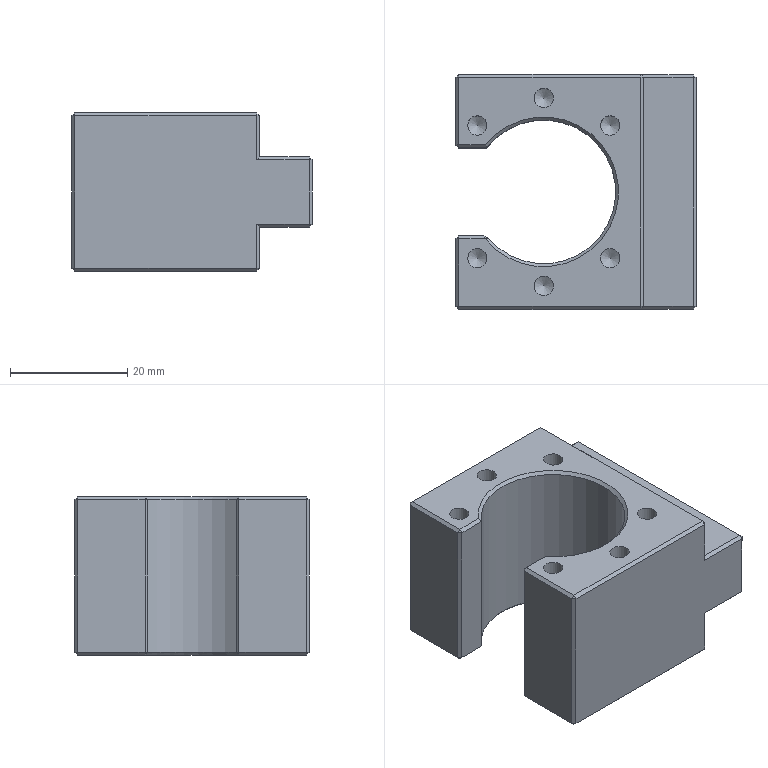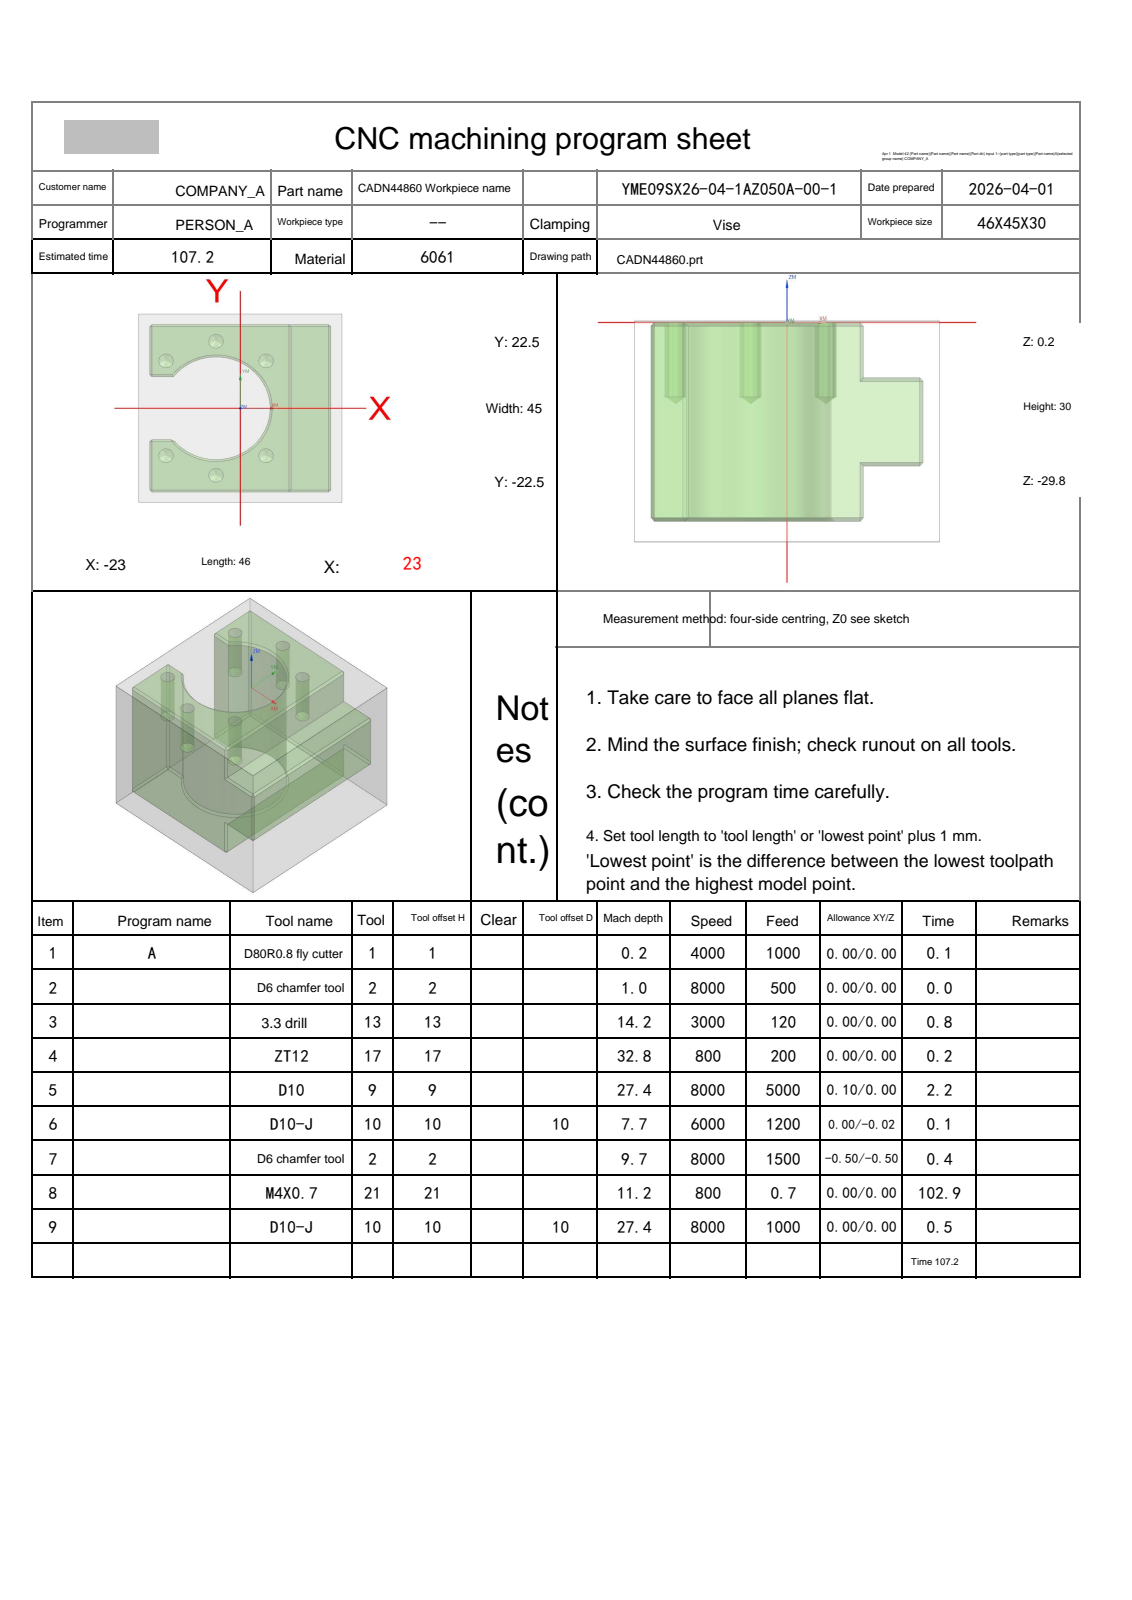NC program | NX | posted by the shop | part box 41 x 40 x 27 mm
Whole program, first 1134 of 1687 lines:
%
O0001
(Machine time: 203.22 MIN)
(===Total Tool:7===)
(T1=D80R0.8 fly cutter  D=80.  R=0.8  D-  H01 Z=-0.   )
(T2=D6 chamfer tool   D=6.   R=0.   D-  H02 Z=-9.5  )
(T13=3.3 drill  D=3.3  DR_a=118 D-  H13 Z=-14.  )
(T17=ZT12   D=12.  DR_a=118 D-  H17 Z=-32.61)
(T9=D10     D=10.  R=0.   D-  H09 Z=-27.2 )
(T10=D10-J  D=10.  R=0.   D10 H10 Z=-27.2 )
(T21=M4X0.7 D=3.3  DR_a=180 D-  H21 Z=-11.  )
G80 G90 G17 G49 G40
G91 G28 Z0
M01
N1 T01 M06
(D80R0.8 fly cutter D=80. R=0.8 H=01 ce=0.00 di=0.00)
G00 G90 G54 X-65.5 Y0.0 M03 S4000
G43 H01 Z20.
M08
Z2.
G01 Z0.0 F1000.
X-60.5
X60.5
X65.5
Z2.
G00 Z20.
G91 G28 Z0.0
M05
M09
G91 G28 Z0.0
M01
N2 T02 M06
(D6 chamfer tool D=6. R=0. H=02 ce=0.00 di=0.00)
G00 G90 G54 X-16.809 Y-11.314 M03 S8000
G43 H02 Z20.
M08
G98 G81 X-16.809 Y-11.314 Z-.8 R1. F500.
X-5.496 Y-16.
X5.818 Y-11.314
X-5.5 Y0.0
X-16.809 Y11.314
X-5.496 Y16.
X5.818 Y11.314
G80
G00 Z20.
G91 G28 Z0.0
M05
M09
G91 G28 Z0.0
M01
N3 T13 M06
(3.3 drill D=3.3 DR_a=118 H=13)
G00 G90 G54 X5.818 Y11.314 M03 S3000
G43 H13 Z20.
M08
G98 G83 X5.818 Y11.314 Z-14. R1. F120. Q2.
X-5.496 Y16.
X-16.809 Y11.314
Y-11.314
X-5.496 Y-16.
X5.818 Y-11.314
G80
G00 Z20.
G91 G28 Z0.0
M05
M09
G91 G28 Z0.0
M01
N4 T17 M06
(ZT12 D=12. DR_a=118 H=17)
G00 G90 G54 X-5.5 Y0.0 M03 S800
G43 H17 Z20.
M08
G98 G83 X-5.5 Y0.0 Z-32.605 R1. F200. Q3.
G80
G00 Z20.
G91 G28 Z0.0
M05
M09
G91 G28 Z0.0
M01
N5 T09 M06
(D10  D=10. R=0. H=09 ce=0.10 di=0.00)
G00 G90 G54 X0.0 Y-25.1 M03 S8000
G43 H09 Z20.
M08
Z.5
G01 X-20. Z.436 F5000.
G02 X-23.606 Y-23.606 Z.424 I0.0 J5.1
G01 X-24.106 Y-23.106 Z.421
G02 X-25.6 Y-19.5 Z.409 I3.606 J3.606
G01 Y-8. Z.372
G02 X-24.106 Y-4.394 Z.359 I5.1 J0.0
G01 X-23.606 Y-3.894 Z.357
G02 X-20. Y-2.4 Z.344 I3.606 J-3.606
G01 X-15.699 Z.331
G02 X-13.545 Y-2.877 Z.323 I0.0 J-5.1
G01 X-12.724 Y-3.26 Z.321
G02 X-10.973 Y-4.601 Z.314 I-2.153 J-4.623
G03 X-.899 Y-5.473 Z.278 I5.473 J4.601
X-.027 Y4.601 Z.242 I-4.601 J5.473
X-10.101 Y5.473 Z.206 I-5.473 J-4.601
X-11.153 Y4.378 Z.201 I4.601 J-5.473
G02 X-15.186 Y2.4 Z.187 I-4.032 J3.122
G01 X-20. Z.171
G02 X-23.606 Y3.894 Z.159 I0.0 J5.1
G01 X-24.106 Y4.394 Z.156
G02 X-25.6 Y8. Z.144 I3.606 J3.606
G01 Y19.5 Z.107
G02 X-24.106 Y23.106 Z.094 I5.1 J0.0
G01 X-23.606 Y23.606 Z.092
G02 X-20. Y25.1 Z.079 I3.606 J-3.606
G01 X20. Z-.048
G02 X23.606 Y23.606 Z-.061 I0.0 J-5.1
G01 X24.106 Y23.106 Z-.063
G02 X25.6 Y19.5 Z-.076 I-3.606 J-3.606
G01 Y-19.5 Z-.2
G02 X24.106 Y-23.106 Z-.213 I-5.1 J0.0
G01 X23.606 Y-23.606 Z-.215
G02 X20. Y-25.1 Z-.228 I-3.606 J3.606
G01 X-20. Z-.355
G02 X-23.606 Y-23.606 Z-.368 I0.0 J5.1
G01 X-24.106 Y-23.106 Z-.37
G02 X-25.6 Y-19.5 Z-.383 I3.606 J3.606
G01 Y-8. Z-.419
G02 X-24.106 Y-4.394 Z-.432 I5.1 J0.0
G01 X-23.606 Y-3.894 Z-.434
G02 X-20. Y-2.4 Z-.447 I3.606 J-3.606
G01 X-15.699 Z-.461
G02 X-13.545 Y-2.877 Z-.468 I0.0 J-5.1
G01 X-12.724 Y-3.26 Z-.471
G02 X-10.973 Y-4.601 Z-.478 I-2.153 J-4.623
G03 X-.899 Y-5.473 Z-.514 I5.473 J4.601
X-.027 Y4.601 Z-.549 I-4.601 J5.473
X-10.101 Y5.473 Z-.585 I-5.473 J-4.601
X-11.153 Y4.378 Z-.59 I4.601 J-5.473
G02 X-15.186 Y2.4 Z-.605 I-4.032 J3.122
G01 X-20. Z-.62
G02 X-23.606 Y3.894 Z-.633 I0.0 J5.1
G01 X-24.106 Y4.394 Z-.635
G02 X-25.6 Y8. Z-.648 I3.606 J3.606
G01 Y19.5 Z-.684
G02 X-24.106 Y23.106 Z-.697 I5.1 J0.0
G01 X-23.606 Y23.606 Z-.699
G02 X-20. Y25.1 Z-.712 I3.606 J-3.606
G01 X20. Z-.84
G02 X23.606 Y23.606 Z-.852 I0.0 J-5.1
G01 X24.106 Y23.106 Z-.855
G02 X25.6 Y19.5 Z-.867 I-3.606 J-3.606
G01 Y-19.5 Z-.991
G02 X24.106 Y-23.106 Z-1.004 I-5.1 J0.0
G01 X23.606 Y-23.606 Z-1.006
G02 X20. Y-25.1 Z-1.019 I-3.606 J3.606
G01 X-20. Z-1.147
G02 X-23.606 Y-23.606 Z-1.159 I0.0 J5.1
G01 X-24.106 Y-23.106 Z-1.162
G02 X-25.6 Y-19.5 Z-1.174 I3.606 J3.606
G01 Y-8. Z-1.211
G02 X-24.106 Y-4.394 Z-1.224 I5.1 J0.0
G01 X-23.606 Y-3.894 Z-1.226
G02 X-20. Y-2.4 Z-1.239 I3.606 J-3.606
G01 X-15.699 Z-1.252
G02 X-13.545 Y-2.877 Z-1.259 I0.0 J-5.1
G01 X-12.724 Y-3.26 Z-1.262
G02 X-10.973 Y-4.601 Z-1.269 I-2.153 J-4.623
G03 X-.899 Y-5.473 Z-1.305 I5.473 J4.601
X-.027 Y4.601 Z-1.341 I-4.601 J5.473
X-10.101 Y5.473 Z-1.377 I-5.473 J-4.601
X-11.153 Y4.378 Z-1.381 I4.601 J-5.473
G02 X-15.186 Y2.4 Z-1.396 I-4.032 J3.122
G01 X-20. Z-1.412
G02 X-23.606 Y3.894 Z-1.424 I0.0 J5.1
G01 X-24.106 Y4.394 Z-1.427
G02 X-25.6 Y8. Z-1.439 I3.606 J3.606
G01 Y19.5 Z-1.476
G02 X-24.106 Y23.106 Z-1.489 I5.1 J0.0
G01 X-23.606 Y23.606 Z-1.491
G02 X-20. Y25.1 Z-1.504 I3.606 J-3.606
G01 X20. Z-1.631
G02 X23.606 Y23.606 Z-1.644 I0.0 J-5.1
G01 X24.106 Y23.106 Z-1.646
G02 X25.6 Y19.5 Z-1.659 I-3.606 J-3.606
G01 Y-19.5 Z-1.783
G02 X24.106 Y-23.106 Z-1.796 I-5.1 J0.0
G01 X23.606 Y-23.606 Z-1.798
G02 X20. Y-25.1 Z-1.811 I-3.606 J3.606
G01 X-20. Z-1.938
G02 X-23.606 Y-23.606 Z-1.951 I0.0 J5.1
G01 X-24.106 Y-23.106 Z-1.953
G02 X-25.6 Y-19.5 Z-1.966 I3.606 J3.606
G01 Y-8. Z-2.002
G02 X-24.106 Y-4.394 Z-2.015 I5.1 J0.0
G01 X-23.606 Y-3.894 Z-2.017
G02 X-20. Y-2.4 Z-2.03 I3.606 J-3.606
G01 X-15.699 Z-2.044
G02 X-13.545 Y-2.877 Z-2.051 I0.0 J-5.1
G01 X-12.724 Y-3.26 Z-2.054
G02 X-10.973 Y-4.601 Z-2.061 I-2.153 J-4.623
G03 X-.899 Y-5.473 Z-2.097 I5.473 J4.601
X-.027 Y4.601 Z-2.132 I-4.601 J5.473
X-10.101 Y5.473 Z-2.168 I-5.473 J-4.601
X-11.153 Y4.378 Z-2.173 I4.601 J-5.473
G02 X-15.186 Y2.4 Z-2.188 I-4.032 J3.122
G01 X-20. Z-2.203
G02 X-23.606 Y3.894 Z-2.216 I0.0 J5.1
G01 X-24.106 Y4.394 Z-2.218
G02 X-25.6 Y8. Z-2.231 I3.606 J3.606
G01 Y19.5 Z-2.267
G02 X-24.106 Y23.106 Z-2.28 I5.1 J0.0
G01 X-23.606 Y23.606 Z-2.282
G02 X-20. Y25.1 Z-2.295 I3.606 J-3.606
G01 X20. Z-2.422
G02 X23.606 Y23.606 Z-2.435 I0.0 J-5.1
G01 X24.106 Y23.106 Z-2.437
G02 X25.6 Y19.5 Z-2.45 I-3.606 J-3.606
G01 Y-19.5 Z-2.574
G02 X24.106 Y-23.106 Z-2.587 I-5.1 J0.0
G01 X23.606 Y-23.606 Z-2.589
G02 X20. Y-25.1 Z-2.602 I-3.606 J3.606
G01 X-20. Z-2.729
G02 X-23.606 Y-23.606 Z-2.742 I0.0 J5.1
G01 X-24.106 Y-23.106 Z-2.744
G02 X-25.6 Y-19.5 Z-2.757 I3.606 J3.606
G01 Y-8. Z-2.794
G02 X-24.106 Y-4.394 Z-2.806 I5.1 J0.0
G01 X-23.606 Y-3.894 Z-2.809
G02 X-20. Y-2.4 Z-2.821 I3.606 J-3.606
G01 X-15.699 Z-2.835
G02 X-13.545 Y-2.877 Z-2.842 I0.0 J-5.1
G01 X-12.724 Y-3.26 Z-2.845
G02 X-10.973 Y-4.601 Z-2.852 I-2.153 J-4.623
G03 X-.899 Y-5.473 Z-2.888 I5.473 J4.601
X-.027 Y4.601 Z-2.924 I-4.601 J5.473
X-10.101 Y5.473 Z-2.959 I-5.473 J-4.601
X-11.153 Y4.378 Z-2.964 I4.601 J-5.473
G02 X-15.186 Y2.4 Z-2.979 I-4.032 J3.122
G01 X-20. Z-2.994
G02 X-23.606 Y3.894 Z-3.007 I0.0 J5.1
G01 X-24.106 Y4.394 Z-3.009
G02 X-25.6 Y8. Z-3.022 I3.606 J3.606
G01 Y19.5 Z-3.059
G02 X-24.106 Y23.106 Z-3.072 I5.1 J0.0
G01 X-23.606 Y23.606 Z-3.074
G02 X-20. Y25.1 Z-3.087 I3.606 J-3.606
G01 X20. Z-3.214
G02 X23.606 Y23.606 Z-3.227 I0.0 J-5.1
G01 X24.106 Y23.106 Z-3.229
G02 X25.6 Y19.5 Z-3.242 I-3.606 J-3.606
G01 Y-19.5 Z-3.366
G02 X24.106 Y-23.106 Z-3.378 I-5.1 J0.0
G01 X23.606 Y-23.606 Z-3.381
G02 X20. Y-25.1 Z-3.393 I-3.606 J3.606
G01 X-20. Z-3.521
G02 X-23.606 Y-23.606 Z-3.534 I0.0 J5.1
G01 X-24.106 Y-23.106 Z-3.536
G02 X-25.6 Y-19.5 Z-3.549 I3.606 J3.606
G01 Y-8. Z-3.585
G02 X-24.106 Y-4.394 Z-3.598 I5.1 J0.0
G01 X-23.606 Y-3.894 Z-3.6
G02 X-20. Y-2.4 Z-3.613 I3.606 J-3.606
G01 X-15.699 Z-3.627
G02 X-13.545 Y-2.877 Z-3.634 I0.0 J-5.1
G01 X-12.724 Y-3.26 Z-3.637
G02 X-10.973 Y-4.601 Z-3.644 I-2.153 J-4.623
G03 X-.899 Y-5.473 Z-3.679 I5.473 J4.601
X-.027 Y4.601 Z-3.715 I-4.601 J5.473
X-10.101 Y5.473 Z-3.751 I-5.473 J-4.601
X-11.153 Y4.378 Z-3.756 I4.601 J-5.473
G02 X-15.186 Y2.4 Z-3.771 I-4.032 J3.122
G01 X-20. Z-3.786
G02 X-23.606 Y3.894 Z-3.799 I0.0 J5.1
G01 X-24.106 Y4.394 Z-3.801
G02 X-25.6 Y8. Z-3.814 I3.606 J3.606
G01 Y19.5 Z-3.85
G02 X-24.106 Y23.106 Z-3.863 I5.1 J0.0
G01 X-23.606 Y23.606 Z-3.865
G02 X-20. Y25.1 Z-3.878 I3.606 J-3.606
G01 X20. Z-4.005
G02 X23.606 Y23.606 Z-4.018 I0.0 J-5.1
G01 X24.106 Y23.106 Z-4.02
G02 X25.6 Y19.5 Z-4.033 I-3.606 J-3.606
G01 Y-19.5 Z-4.157
G02 X24.106 Y-23.106 Z-4.17 I-5.1 J0.0
G01 X23.606 Y-23.606 Z-4.172
G02 X20. Y-25.1 Z-4.185 I-3.606 J3.606
G01 X-20. Z-4.312
G02 X-23.606 Y-23.606 Z-4.325 I0.0 J5.1
G01 X-24.106 Y-23.106 Z-4.327
G02 X-25.6 Y-19.5 Z-4.34 I3.606 J3.606
G01 Y-8. Z-4.377
G02 X-24.106 Y-4.394 Z-4.389 I5.1 J0.0
G01 X-23.606 Y-3.894 Z-4.392
G02 X-20. Y-2.4 Z-4.404 I3.606 J-3.606
G01 X-15.699 Z-4.418
G02 X-13.545 Y-2.877 Z-4.425 I0.0 J-5.1
G01 X-12.724 Y-3.26 Z-4.428
G02 X-10.973 Y-4.601 Z-4.435 I-2.153 J-4.623
G03 X-.899 Y-5.473 Z-4.471 I5.473 J4.601
X-.027 Y4.601 Z-4.507 I-4.601 J5.473
X-10.101 Y5.473 Z-4.542 I-5.473 J-4.601
X-11.153 Y4.378 Z-4.547 I4.601 J-5.473
G02 X-15.186 Y2.4 Z-4.562 I-4.032 J3.122
G01 X-20. Z-4.577
G02 X-23.606 Y3.894 Z-4.59 I0.0 J5.1
G01 X-24.106 Y4.394 Z-4.592
G02 X-25.6 Y8. Z-4.605 I3.606 J3.606
G01 Y19.5 Z-4.642
G02 X-24.106 Y23.106 Z-4.654 I5.1 J0.0
G01 X-23.606 Y23.606 Z-4.657
G02 X-20. Y25.1 Z-4.669 I3.606 J-3.606
G01 X20. Z-4.797
G02 X23.606 Y23.606 Z-4.809 I0.0 J-5.1
G01 X24.106 Y23.106 Z-4.812
G02 X25.6 Y19.5 Z-4.824 I-3.606 J-3.606
G01 Y-19.5 Z-4.949
G02 X24.106 Y-23.106 Z-4.961 I-5.1 J0.0
G01 X23.606 Y-23.606 Z-4.964
G02 X20. Y-25.1 Z-4.976 I-3.606 J3.606
G01 X-20. Z-5.104
G02 X-23.606 Y-23.606 Z-5.116 I0.0 J5.1
G01 X-24.106 Y-23.106 Z-5.119
G02 X-25.6 Y-19.5 Z-5.131 I3.606 J3.606
G01 Y-8. Z-5.168
G02 X-24.106 Y-4.394 Z-5.181 I5.1 J0.0
G01 X-23.606 Y-3.894 Z-5.183
G02 X-20. Y-2.4 Z-5.196 I3.606 J-3.606
G01 X-15.699 Z-5.209
G02 X-13.545 Y-2.877 Z-5.217 I0.0 J-5.1
G01 X-12.724 Y-3.26 Z-5.219
G02 X-10.973 Y-4.601 Z-5.226 I-2.153 J-4.623
G03 X-.899 Y-5.473 Z-5.262 I5.473 J4.601
X-.027 Y4.601 Z-5.298 I-4.601 J5.473
X-10.101 Y5.473 Z-5.334 I-5.473 J-4.601
X-11.153 Y4.378 Z-5.339 I4.601 J-5.473
G02 X-15.186 Y2.4 Z-5.353 I-4.032 J3.122
G01 X-20. Z-5.369
G02 X-23.606 Y3.894 Z-5.381 I0.0 J5.1
G01 X-24.106 Y4.394 Z-5.384
G02 X-25.6 Y8. Z-5.396 I3.606 J3.606
G01 Y19.5 Z-5.433
G02 X-24.106 Y23.106 Z-5.446 I5.1 J0.0
G01 X-23.606 Y23.606 Z-5.448
G02 X-20. Y25.1 Z-5.461 I3.606 J-3.606
G01 X20. Z-5.588
G02 X23.606 Y23.606 Z-5.601 I0.0 J-5.1
G01 X24.106 Y23.106 Z-5.603
G02 X25.6 Y19.5 Z-5.616 I-3.606 J-3.606
G01 Y-19.5 Z-5.74
G02 X24.106 Y-23.106 Z-5.753 I-5.1 J0.0
G01 X23.606 Y-23.606 Z-5.755
G02 X20. Y-25.1 Z-5.768 I-3.606 J3.606
G01 X-20. Z-5.895
G02 X-23.606 Y-23.606 Z-5.908 I0.0 J5.1
G01 X-24.106 Y-23.106 Z-5.91
G02 X-25.6 Y-19.5 Z-5.923 I3.606 J3.606
G01 Y-8. Z-5.959
G02 X-24.106 Y-4.394 Z-5.972 I5.1 J0.0
G01 X-23.606 Y-3.894 Z-5.974
G02 X-20. Y-2.4 Z-5.987 I3.606 J-3.606
G01 X-15.699 Z-6.001
G02 X-13.545 Y-2.877 Z-6.008 I0.0 J-5.1
G01 X-12.724 Y-3.26 Z-6.011
G02 X-10.973 Y-4.601 Z-6.018 I-2.153 J-4.623
G03 X-.899 Y-5.473 Z-6.054 I5.473 J4.601
X-.027 Y4.601 Z-6.089 I-4.601 J5.473
X-10.101 Y5.473 Z-6.125 I-5.473 J-4.601
X-11.153 Y4.378 Z-6.13 I4.601 J-5.473
G02 X-15.186 Y2.4 Z-6.145 I-4.032 J3.122
G01 X-20. Z-6.16
G02 X-23.606 Y3.894 Z-6.173 I0.0 J5.1
G01 X-24.106 Y4.394 Z-6.175
G02 X-25.6 Y8. Z-6.188 I3.606 J3.606
G01 Y19.5 Z-6.224
G02 X-24.106 Y23.106 Z-6.237 I5.1 J0.0
G01 X-23.606 Y23.606 Z-6.239
G02 X-20. Y25.1 Z-6.252 I3.606 J-3.606
G01 X20. Z-6.38
G02 X23.606 Y23.606 Z-6.392 I0.0 J-5.1
G01 X24.106 Y23.106 Z-6.395
G02 X25.6 Y19.5 Z-6.407 I-3.606 J-3.606
G01 Y-19.5 Z-6.531
G02 X24.106 Y-23.106 Z-6.544 I-5.1 J0.0
G01 X23.606 Y-23.606 Z-6.546
G02 X20. Y-25.1 Z-6.559 I-3.606 J3.606
G01 X-20. Z-6.687
G02 X-23.606 Y-23.606 Z-6.699 I0.0 J5.1
G01 X-24.106 Y-23.106 Z-6.702
G02 X-25.6 Y-19.5 Z-6.714 I3.606 J3.606
G01 Y-8. Z-6.751
G02 X-24.106 Y-4.394 Z-6.764 I5.1 J0.0
G01 X-23.606 Y-3.894 Z-6.766
G02 X-20. Y-2.4 Z-6.779 I3.606 J-3.606
G01 X-15.699 Z-6.792
G02 X-13.545 Y-2.877 Z-6.799 I0.0 J-5.1
G01 X-12.724 Y-3.26 Z-6.802
G02 X-10.973 Y-4.601 Z-6.809 I-2.153 J-4.623
G03 X-.899 Y-5.473 Z-6.845 I5.473 J4.601
X-.027 Y4.601 Z-6.881 I-4.601 J5.473
X-10.101 Y5.473 Z-6.917 I-5.473 J-4.601
X-11.153 Y4.378 Z-6.921 I4.601 J-5.473
G02 X-15.186 Y2.4 Z-6.936 I-4.032 J3.122
G01 X-20. Z-6.952
G02 X-23.606 Y3.894 Z-6.964 I0.0 J5.1
G01 X-24.106 Y4.394 Z-6.967
G02 X-25.6 Y8. Z-6.979 I3.606 J3.606
G01 Y19.5 Z-7.016
G02 X-24.106 Y23.106 Z-7.029 I5.1 J0.0
G01 X-23.606 Y23.606 Z-7.031
G02 X-20. Y25.1 Z-7.044 I3.606 J-3.606
G01 X20. Z-7.171
G02 X23.606 Y23.606 Z-7.184 I0.0 J-5.1
G01 X24.106 Y23.106 Z-7.186
G02 X25.6 Y19.5 Z-7.199 I-3.606 J-3.606
G01 Y-19.5 Z-7.323
G02 X24.106 Y-23.106 Z-7.336 I-5.1 J0.0
G01 X23.606 Y-23.606 Z-7.338
G02 X20. Y-25.1 Z-7.351 I-3.606 J3.606
G01 X-20. Z-7.478
G02 X-23.606 Y-23.606 Z-7.491 I0.0 J5.1
G01 X-24.106 Y-23.106 Z-7.493
G02 X-25.6 Y-19.5 Z-7.506 I3.606 J3.606
G01 Y-8. Z-7.542
G02 X-24.106 Y-4.394 Z-7.555 I5.1 J0.0
G01 X-23.606 Y-3.894 Z-7.557
G02 X-20. Y-2.4 Z-7.57 I3.606 J-3.606
G01 X-15.699 Z-7.584
G02 X-13.545 Y-2.877 Z-7.591 I0.0 J-5.1
G01 X-12.724 Y-3.26 Z-7.594
G02 X-10.973 Y-4.601 Z-7.601 I-2.153 J-4.623
G03 X-.899 Y-5.473 Z-7.637 I5.473 J4.601
X-.027 Y4.601 Z-7.672 I-4.601 J5.473
X-10.101 Y5.473 Z-7.708 I-5.473 J-4.601
X-11.153 Y4.378 Z-7.713 I4.601 J-5.473
G02 X-15.186 Y2.4 Z-7.728 I-4.032 J3.122
G01 X-20. Z-7.743
G02 X-23.606 Y3.894 Z-7.756 I0.0 J5.1
G01 X-24.106 Y4.394 Z-7.758
G02 X-25.6 Y8. Z-7.771 I3.606 J3.606
G01 Y19.5 Z-7.807
G02 X-24.106 Y23.106 Z-7.82 I5.1 J0.0
G01 X-23.606 Y23.606 Z-7.822
G02 X-20. Y25.1 Z-7.835 I3.606 J-3.606
G01 X20. Z-7.962
G02 X23.606 Y23.606 Z-7.975 I0.0 J-5.1
G01 X24.106 Y23.106 Z-7.977
G02 X25.6 Y19.5 Z-7.99 I-3.606 J-3.606
G01 Y-19.5 Z-8.114
G02 X24.106 Y-23.106 Z-8.127 I-5.1 J0.0
G01 X23.606 Y-23.606 Z-8.129
G02 X20. Y-25.1 Z-8.142 I-3.606 J3.606
G01 X-20. Z-8.269
G02 X-23.606 Y-23.606 Z-8.282 I0.0 J5.1
G01 X-24.106 Y-23.106 Z-8.284
G02 X-25.6 Y-19.5 Z-8.297 I3.606 J3.606
G01 Y-8. Z-8.334
G02 X-24.106 Y-4.394 Z-8.346 I5.1 J0.0
G01 X-23.606 Y-3.894 Z-8.349
G02 X-20. Y-2.4 Z-8.361 I3.606 J-3.606
G01 X-15.699 Z-8.375
G02 X-13.545 Y-2.877 Z-8.382 I0.0 J-5.1
G01 X-12.724 Y-3.26 Z-8.385
G02 X-10.973 Y-4.601 Z-8.392 I-2.153 J-4.623
G03 X-.899 Y-5.473 Z-8.428 I5.473 J4.601
X-.027 Y4.601 Z-8.464 I-4.601 J5.473
X-10.101 Y5.473 Z-8.499 I-5.473 J-4.601
X-11.153 Y4.378 Z-8.504 I4.601 J-5.473
G02 X-15.186 Y2.4 Z-8.519 I-4.032 J3.122
G01 X-20. Z-8.534
G02 X-23.606 Y3.894 Z-8.547 I0.0 J5.1
G01 X-24.106 Y4.394 Z-8.549
G02 X-25.6 Y8. Z-8.562 I3.606 J3.606
G01 Y19.5 Z-8.599
G02 X-24.106 Y23.106 Z-8.612 I5.1 J0.0
G01 X-23.606 Y23.606 Z-8.614
G02 X-20. Y25.1 Z-8.627 I3.606 J-3.606
G01 X20. Z-8.754
G02 X23.606 Y23.606 Z-8.767 I0.0 J-5.1
G01 X24.106 Y23.106 Z-8.769
G02 X25.6 Y19.5 Z-8.782 I-3.606 J-3.606
G01 Y-19.5 Z-8.906
G02 X24.106 Y-23.106 Z-8.918 I-5.1 J0.0
G01 X23.606 Y-23.606 Z-8.921
G02 X20. Y-25.1 Z-8.933 I-3.606 J3.606
G01 X-20. Z-9.061
G02 X-23.606 Y-23.606 Z-9.074 I0.0 J5.1
G01 X-24.106 Y-23.106 Z-9.076
G02 X-25.6 Y-19.5 Z-9.089 I3.606 J3.606
G01 Y-8. Z-9.125
G02 X-24.106 Y-4.394 Z-9.138 I5.1 J0.0
G01 X-23.606 Y-3.894 Z-9.14
G02 X-20. Y-2.4 Z-9.153 I3.606 J-3.606
G01 X-15.699 Z-9.167
G02 X-13.545 Y-2.877 Z-9.174 I0.0 J-5.1
G01 X-12.724 Y-3.26 Z-9.177
G02 X-10.973 Y-4.601 Z-9.184 I-2.153 J-4.623
G03 X-.899 Y-5.473 Z-9.219 I5.473 J4.601
X-.027 Y4.601 Z-9.255 I-4.601 J5.473
X-10.101 Y5.473 Z-9.291 I-5.473 J-4.601
X-11.153 Y4.378 Z-9.296 I4.601 J-5.473
G02 X-15.186 Y2.4 Z-9.311 I-4.032 J3.122
G01 X-20. Z-9.326
G02 X-23.606 Y3.894 Z-9.339 I0.0 J5.1
G01 X-24.106 Y4.394 Z-9.341
G02 X-25.6 Y8. Z-9.354 I3.606 J3.606
G01 Y19.5 Z-9.39
G02 X-24.106 Y23.106 Z-9.403 I5.1 J0.0
G01 X-23.606 Y23.606 Z-9.405
G02 X-20. Y25.1 Z-9.418 I3.606 J-3.606
G01 X20. Z-9.545
G02 X23.606 Y23.606 Z-9.558 I0.0 J-5.1
G01 X24.106 Y23.106 Z-9.56
G02 X25.6 Y19.5 Z-9.573 I-3.606 J-3.606
G01 Y-19.5 Z-9.697
G02 X24.106 Y-23.106 Z-9.71 I-5.1 J0.0
G01 X23.606 Y-23.606 Z-9.712
G02 X20. Y-25.1 Z-9.725 I-3.606 J3.606
G01 X-20. Z-9.852
G02 X-23.606 Y-23.606 Z-9.865 I0.0 J5.1
G01 X-24.106 Y-23.106 Z-9.867
G02 X-25.6 Y-19.5 Z-9.88 I3.606 J3.606
G01 Y-8. Z-9.917
G02 X-24.106 Y-4.394 Z-9.929 I5.1 J0.0
G01 X-23.606 Y-3.894 Z-9.932
G02 X-20. Y-2.4 Z-9.944 I3.606 J-3.606
G01 X-15.699 Z-9.958
G02 X-13.545 Y-2.877 Z-9.965 I0.0 J-5.1
G01 X-12.724 Y-3.26 Z-9.968
G02 X-10.973 Y-4.601 Z-9.975 I-2.153 J-4.623
G03 X-.899 Y-5.473 Z-10.011 I5.473 J4.601
X-.027 Y4.601 Z-10.047 I-4.601 J5.473
X-10.101 Y5.473 Z-10.082 I-5.473 J-4.601
X-11.153 Y4.378 Z-10.087 I4.601 J-5.473
G02 X-15.186 Y2.4 Z-10.102 I-4.032 J3.122
G01 X-20. Z-10.117
G02 X-23.606 Y3.894 Z-10.13 I0.0 J5.1
G01 X-24.106 Y4.394 Z-10.132
G02 X-25.6 Y8. Z-10.145 I3.606 J3.606
G01 Y19.5 Z-10.182
G02 X-24.106 Y23.106 Z-10.194 I5.1 J0.0
G01 X-23.606 Y23.606 Z-10.197
G02 X-20. Y25.1 Z-10.209 I3.606 J-3.606
G01 X20. Z-10.337
G02 X23.606 Y23.606 Z-10.349 I0.0 J-5.1
G01 X24.106 Y23.106 Z-10.352
G02 X25.6 Y19.5 Z-10.364 I-3.606 J-3.606
G01 Y-19.5 Z-10.489
G02 X24.106 Y-23.106 Z-10.501 I-5.1 J0.0
G01 X23.606 Y-23.606 Z-10.504
G02 X20. Y-25.1 Z-10.516 I-3.606 J3.606
G01 X-20. Z-10.644
G02 X-23.606 Y-23.606 Z-10.656 I0.0 J5.1
G01 X-24.106 Y-23.106 Z-10.659
G02 X-25.6 Y-19.5 Z-10.671 I3.606 J3.606
G01 Y-8. Z-10.708
G02 X-24.106 Y-4.394 Z-10.721 I5.1 J0.0
G01 X-23.606 Y-3.894 Z-10.723
G02 X-20. Y-2.4 Z-10.736 I3.606 J-3.606
G01 X-15.699 Z-10.749
G02 X-13.545 Y-2.877 Z-10.757 I0.0 J-5.1
G01 X-12.724 Y-3.26 Z-10.759
G02 X-10.973 Y-4.601 Z-10.766 I-2.153 J-4.623
G03 X-.899 Y-5.473 Z-10.802 I5.473 J4.601
X-.027 Y4.601 Z-10.838 I-4.601 J5.473
X-10.101 Y5.473 Z-10.874 I-5.473 J-4.601
X-11.153 Y4.378 Z-10.879 I4.601 J-5.473
G02 X-15.186 Y2.4 Z-10.893 I-4.032 J3.122
G01 X-20. Z-10.909
G02 X-23.606 Y3.894 Z-10.921 I0.0 J5.1
G01 X-24.106 Y4.394 Z-10.924
G02 X-25.6 Y8. Z-10.936 I3.606 J3.606
G01 Y19.5 Z-10.973
G02 X-24.106 Y23.106 Z-10.986 I5.1 J0.0
G01 X-23.606 Y23.606 Z-10.988
G02 X-20. Y25.1 Z-11.001 I3.606 J-3.606
G01 X20. Z-11.128
G02 X23.606 Y23.606 Z-11.141 I0.0 J-5.1
G01 X24.106 Y23.106 Z-11.143
G02 X25.6 Y19.5 Z-11.156 I-3.606 J-3.606
G01 Y-19.5 Z-11.28
G02 X24.106 Y-23.106 Z-11.293 I-5.1 J0.0
G01 X23.606 Y-23.606 Z-11.295
G02 X20. Y-25.1 Z-11.308 I-3.606 J3.606
G01 X-20. Z-11.435
G02 X-23.606 Y-23.606 Z-11.448 I0.0 J5.1
G01 X-24.106 Y-23.106 Z-11.45
G02 X-25.6 Y-19.5 Z-11.463 I3.606 J3.606
G01 Y-8. Z-11.499
G02 X-24.106 Y-4.394 Z-11.512 I5.1 J0.0
G01 X-23.606 Y-3.894 Z-11.514
G02 X-20. Y-2.4 Z-11.527 I3.606 J-3.606
G01 X-15.699 Z-11.541
G02 X-13.545 Y-2.877 Z-11.548 I0.0 J-5.1
G01 X-12.724 Y-3.26 Z-11.551
G02 X-10.973 Y-4.601 Z-11.558 I-2.153 J-4.623
G03 X-.899 Y-5.473 Z-11.594 I5.473 J4.601
X-.027 Y4.601 Z-11.629 I-4.601 J5.473
X-10.101 Y5.473 Z-11.665 I-5.473 J-4.601
X-11.153 Y4.378 Z-11.67 I4.601 J-5.473
G02 X-15.186 Y2.4 Z-11.685 I-4.032 J3.122
G01 X-20. Z-11.7
G02 X-23.606 Y3.894 Z-11.713 I0.0 J5.1
G01 X-24.106 Y4.394 Z-11.715
G02 X-25.6 Y8. Z-11.728 I3.606 J3.606
G01 Y19.5 Z-11.764
G02 X-24.106 Y23.106 Z-11.777 I5.1 J0.0
G01 X-23.606 Y23.606 Z-11.779
G02 X-20. Y25.1 Z-11.792 I3.606 J-3.606
G01 X20. Z-11.92
G02 X23.606 Y23.606 Z-11.932 I0.0 J-5.1
G01 X24.106 Y23.106 Z-11.935
G02 X25.6 Y19.5 Z-11.947 I-3.606 J-3.606
G01 Y-19.5 Z-12.071
G02 X24.106 Y-23.106 Z-12.084 I-5.1 J0.0
G01 X23.606 Y-23.606 Z-12.086
G02 X20. Y-25.1 Z-12.099 I-3.606 J3.606
G01 X-20. Z-12.227
G02 X-23.606 Y-23.606 Z-12.239 I0.0 J5.1
G01 X-24.106 Y-23.106 Z-12.242
G02 X-25.6 Y-19.5 Z-12.254 I3.606 J3.606
G01 Y-8. Z-12.291
G02 X-24.106 Y-4.394 Z-12.304 I5.1 J0.0
G01 X-23.606 Y-3.894 Z-12.306
G02 X-20. Y-2.4 Z-12.319 I3.606 J-3.606
G01 X-15.699 Z-12.332
G02 X-13.545 Y-2.877 Z-12.339 I0.0 J-5.1
G01 X-12.724 Y-3.26 Z-12.342
G02 X-10.973 Y-4.601 Z-12.349 I-2.153 J-4.623
G03 X-.899 Y-5.473 Z-12.385 I5.473 J4.601
X-.027 Y4.601 Z-12.421 I-4.601 J5.473
X-10.101 Y5.473 Z-12.457 I-5.473 J-4.601
X-11.153 Y4.378 Z-12.461 I4.601 J-5.473
G02 X-15.186 Y2.4 Z-12.476 I-4.032 J3.122
G01 X-20. Z-12.492
G02 X-23.606 Y3.894 Z-12.504 I0.0 J5.1
G01 X-24.106 Y4.394 Z-12.507
G02 X-25.6 Y8. Z-12.519 I3.606 J3.606
G01 Y19.5 Z-12.556
G02 X-24.106 Y23.106 Z-12.569 I5.1 J0.0
G01 X-23.606 Y23.606 Z-12.571
G02 X-20. Y25.1 Z-12.584 I3.606 J-3.606
G01 X20. Z-12.711
G02 X23.606 Y23.606 Z-12.724 I0.0 J-5.1
G01 X24.106 Y23.106 Z-12.726
G02 X25.6 Y19.5 Z-12.739 I-3.606 J-3.606
G01 Y-19.5 Z-12.863
G02 X24.106 Y-23.106 Z-12.876 I-5.1 J0.0
G01 X23.606 Y-23.606 Z-12.878
G02 X20. Y-25.1 Z-12.891 I-3.606 J3.606
G01 X-20. Z-13.018
G02 X-23.606 Y-23.606 Z-13.031 I0.0 J5.1
G01 X-24.106 Y-23.106 Z-13.033
G02 X-25.6 Y-19.5 Z-13.046 I3.606 J3.606
G01 Y-8. Z-13.082
G02 X-24.106 Y-4.394 Z-13.095 I5.1 J0.0
G01 X-23.606 Y-3.894 Z-13.097
G02 X-20. Y-2.4 Z-13.11 I3.606 J-3.606
G01 X-15.699 Z-13.124
G02 X-13.545 Y-2.877 Z-13.131 I0.0 J-5.1
G01 X-12.724 Y-3.26 Z-13.134
G02 X-10.973 Y-4.601 Z-13.141 I-2.153 J-4.623
G03 X-.899 Y-5.473 Z-13.177 I5.473 J4.601
X-.027 Y4.601 Z-13.212 I-4.601 J5.473
X-10.101 Y5.473 Z-13.248 I-5.473 J-4.601
X-11.153 Y4.378 Z-13.253 I4.601 J-5.473
G02 X-15.186 Y2.4 Z-13.268 I-4.032 J3.122
G01 X-20. Z-13.283
G02 X-23.606 Y3.894 Z-13.296 I0.0 J5.1
G01 X-24.106 Y4.394 Z-13.298
G02 X-25.6 Y8. Z-13.311 I3.606 J3.606
G01 Y19.5 Z-13.347
G02 X-24.106 Y23.106 Z-13.36 I5.1 J0.0
G01 X-23.606 Y23.606 Z-13.362
G02 X-20. Y25.1 Z-13.375 I3.606 J-3.606
G01 X20. Z-13.502
G02 X23.606 Y23.606 Z-13.515 I0.0 J-5.1
G01 X24.106 Y23.106 Z-13.517
G02 X25.6 Y19.5 Z-13.53 I-3.606 J-3.606
G01 Y-19.5 Z-13.654
G02 X24.106 Y-23.106 Z-13.667 I-5.1 J0.0
G01 X23.606 Y-23.606 Z-13.669
G02 X20. Y-25.1 Z-13.682 I-3.606 J3.606
G01 X-20. Z-13.809
G02 X-23.606 Y-23.606 Z-13.822 I0.0 J5.1
G01 X-24.106 Y-23.106 Z-13.824
G02 X-25.6 Y-19.5 Z-13.837 I3.606 J3.606
G01 Y-8. Z-13.874
G02 X-24.106 Y-4.394 Z-13.886 I5.1 J0.0
G01 X-23.606 Y-3.894 Z-13.889
G02 X-20. Y-2.4 Z-13.901 I3.606 J-3.606
G01 X-15.699 Z-13.915
G02 X-13.545 Y-2.877 Z-13.922 I0.0 J-5.1
G01 X-12.724 Y-3.26 Z-13.925
G02 X-10.973 Y-4.601 Z-13.932 I-2.153 J-4.623
G03 X-.899 Y-5.473 Z-13.968 I5.473 J4.601
X-.027 Y4.601 Z-14.004 I-4.601 J5.473
X-10.101 Y5.473 Z-14.039 I-5.473 J-4.601
X-11.153 Y4.378 Z-14.044 I4.601 J-5.473
G02 X-15.186 Y2.4 Z-14.059 I-4.032 J3.122
G01 X-20. Z-14.074
G02 X-23.606 Y3.894 Z-14.087 I0.0 J5.1
G01 X-24.106 Y4.394 Z-14.089
G02 X-25.6 Y8. Z-14.102 I3.606 J3.606
G01 Y19.5 Z-14.139
G02 X-24.106 Y23.106 Z-14.152 I5.1 J0.0
G01 X-23.606 Y23.606 Z-14.154
G02 X-20. Y25.1 Z-14.167 I3.606 J-3.606
G01 X20. Z-14.294
G02 X23.606 Y23.606 Z-14.307 I0.0 J-5.1
G01 X24.106 Y23.106 Z-14.309
G02 X25.6 Y19.5 Z-14.322 I-3.606 J-3.606
G01 Y-19.5 Z-14.446
G02 X24.106 Y-23.106 Z-14.458 I-5.1 J0.0
G01 X23.606 Y-23.606 Z-14.461
G02 X20. Y-25.1 Z-14.473 I-3.606 J3.606
G01 X-20. Z-14.601
G02 X-23.606 Y-23.606 Z-14.614 I0.0 J5.1
G01 X-24.106 Y-23.106 Z-14.616
G02 X-25.6 Y-19.5 Z-14.629 I3.606 J3.606
G01 Y-8. Z-14.665
G02 X-24.106 Y-4.394 Z-14.678 I5.1 J0.0
G01 X-23.606 Y-3.894 Z-14.68
G02 X-20. Y-2.4 Z-14.693 I3.606 J-3.606
G01 X-15.699 Z-14.707
G02 X-13.545 Y-2.877 Z-14.714 I0.0 J-5.1
G01 X-12.724 Y-3.26 Z-14.717
G02 X-10.973 Y-4.601 Z-14.724 I-2.153 J-4.623
G03 X-.899 Y-5.473 Z-14.759 I5.473 J4.601
X-.027 Y4.601 Z-14.795 I-4.601 J5.473
X-10.101 Y5.473 Z-14.831 I-5.473 J-4.601
X-11.153 Y4.378 Z-14.836 I4.601 J-5.473
G02 X-15.186 Y2.4 Z-14.851 I-4.032 J3.122
G01 X-20. Z-14.866
G02 X-23.606 Y3.894 Z-14.879 I0.0 J5.1
G01 X-24.106 Y4.394 Z-14.881
G02 X-25.6 Y8. Z-14.894 I3.606 J3.606
G01 Y19.5 Z-14.93
G02 X-24.106 Y23.106 Z-14.943 I5.1 J0.0
G01 X-23.606 Y23.606 Z-14.945
G02 X-20. Y25.1 Z-14.958 I3.606 J-3.606
G01 X20. Z-15.085
G02 X23.606 Y23.606 Z-15.098 I0.0 J-5.1
G01 X24.106 Y23.106 Z-15.1
G02 X25.6 Y19.5 Z-15.113 I-3.606 J-3.606
G01 Y-19.5 Z-15.237
G02 X24.106 Y-23.106 Z-15.25 I-5.1 J0.0
G01 X23.606 Y-23.606 Z-15.252
G02 X20. Y-25.1 Z-15.265 I-3.606 J3.606
G01 X-20. Z-15.392
G02 X-23.606 Y-23.606 Z-15.405 I0.0 J5.1
G01 X-24.106 Y-23.106 Z-15.407
G02 X-25.6 Y-19.5 Z-15.42 I3.606 J3.606
G01 Y-8. Z-15.457
G02 X-24.106 Y-4.394 Z-15.469 I5.1 J0.0
G01 X-23.606 Y-3.894 Z-15.472
G02 X-20. Y-2.4 Z-15.484 I3.606 J-3.606
G01 X-15.699 Z-15.498
G02 X-13.545 Y-2.877 Z-15.505 I0.0 J-5.1
G01 X-12.724 Y-3.26 Z-15.508
G02 X-10.973 Y-4.601 Z-15.515 I-2.153 J-4.623
G03 X-.899 Y-5.473 Z-15.551 I5.473 J4.601
X-.027 Y4.601 Z-15.587 I-4.601 J5.473
X-10.101 Y5.473 Z-15.622 I-5.473 J-4.601
X-11.153 Y4.378 Z-15.627 I4.601 J-5.473
G02 X-15.186 Y2.4 Z-15.642 I-4.032 J3.122
G01 X-20. Z-15.657
G02 X-23.606 Y3.894 Z-15.67 I0.0 J5.1
G01 X-24.106 Y4.394 Z-15.672
G02 X-25.6 Y8. Z-15.685 I3.606 J3.606
G01 Y19.5 Z-15.722
G02 X-24.106 Y23.106 Z-15.734 I5.1 J0.0
G01 X-23.606 Y23.606 Z-15.737
G02 X-20. Y25.1 Z-15.749 I3.606 J-3.606
G01 X20. Z-15.877
G02 X23.606 Y23.606 Z-15.889 I0.0 J-5.1
G01 X24.106 Y23.106 Z-15.892
G02 X25.6 Y19.5 Z-15.904 I-3.606 J-3.606
G01 Y-19.5 Z-16.029
G02 X24.106 Y-23.106 Z-16.041 I-5.1 J0.0
G01 X23.606 Y-23.606 Z-16.044
G02 X20. Y-25.1 Z-16.056 I-3.606 J3.606
G01 X-20. Z-16.184
G02 X-23.606 Y-23.606 Z-16.196 I0.0 J5.1
G01 X-24.106 Y-23.106 Z-16.199
G02 X-25.6 Y-19.5 Z-16.211 I3.606 J3.606
G01 Y-8. Z-16.248
G02 X-24.106 Y-4.394 Z-16.261 I5.1 J0.0
G01 X-23.606 Y-3.894 Z-16.263
G02 X-20. Y-2.4 Z-16.276 I3.606 J-3.606
G01 X-15.699 Z-16.289
G02 X-13.545 Y-2.877 Z-16.297 I0.0 J-5.1
G01 X-12.724 Y-3.26 Z-16.299
G02 X-10.973 Y-4.601 Z-16.306 I-2.153 J-4.623
G03 X-.899 Y-5.473 Z-16.342 I5.473 J4.601
X-.027 Y4.601 Z-16.378 I-4.601 J5.473
X-10.101 Y5.473 Z-16.414 I-5.473 J-4.601
X-11.153 Y4.378 Z-16.419 I4.601 J-5.473
G02 X-15.186 Y2.4 Z-16.433 I-4.032 J3.122
G01 X-20. Z-16.449
G02 X-23.606 Y3.894 Z-16.461 I0.0 J5.1
G01 X-24.106 Y4.394 Z-16.464
G02 X-25.6 Y8. Z-16.476 I3.606 J3.606
G01 Y19.5 Z-16.513
G02 X-24.106 Y23.106 Z-16.526 I5.1 J0.0
G01 X-23.606 Y23.606 Z-16.528
G02 X-20. Y25.1 Z-16.541 I3.606 J-3.606
G01 X20. Z-16.668
G02 X23.606 Y23.606 Z-16.681 I0.0 J-5.1
G01 X24.106 Y23.106 Z-16.683
G02 X25.6 Y19.5 Z-16.696 I-3.606 J-3.606
G01 Y-19.5 Z-16.82
G02 X24.106 Y-23.106 Z-16.833 I-5.1 J0.0
G01 X23.606 Y-23.606 Z-16.835
G02 X20. Y-25.1 Z-16.848 I-3.606 J3.606
G01 X-20. Z-16.975
G02 X-23.606 Y-23.606 Z-16.988 I0.0 J5.1
G01 X-24.106 Y-23.106 Z-16.99
G02 X-25.6 Y-19.5 Z-17.003 I3.606 J3.606
G01 Y-8. Z-17.039
G02 X-24.106 Y-4.394 Z-17.052 I5.1 J0.0
G01 X-23.606 Y-3.894 Z-17.054
G02 X-20. Y-2.4 Z-17.067 I3.606 J-3.606
G01 X-15.699 Z-17.081
G02 X-13.545 Y-2.877 Z-17.088 I0.0 J-5.1
G01 X-12.724 Y-3.26 Z-17.091
G02 X-10.973 Y-4.601 Z-17.098 I-2.153 J-4.623
G03 X-.899 Y-5.473 Z-17.134 I5.473 J4.601
X-.027 Y4.601 Z-17.169 I-4.601 J5.473
X-10.101 Y5.473 Z-17.205 I-5.473 J-4.601
X-11.153 Y4.378 Z-17.21 I4.601 J-5.473
G02 X-15.186 Y2.4 Z-17.225 I-4.032 J3.122
G01 X-20. Z-17.24
G02 X-23.606 Y3.894 Z-17.253 I0.0 J5.1
G01 X-24.106 Y4.394 Z-17.255
G02 X-25.6 Y8. Z-17.268 I3.606 J3.606
G01 Y19.5 Z-17.304
G02 X-24.106 Y23.106 Z-17.317 I5.1 J0.0
G01 X-23.606 Y23.606 Z-17.319
G02 X-20. Y25.1 Z-17.332 I3.606 J-3.606
G01 X20. Z-17.46
G02 X23.606 Y23.606 Z-17.472 I0.0 J-5.1
G01 X24.106 Y23.106 Z-17.475
G02 X25.6 Y19.5 Z-17.487 I-3.606 J-3.606
G01 Y-19.5 Z-17.611
G02 X24.106 Y-23.106 Z-17.624 I-5.1 J0.0
G01 X23.606 Y-23.606 Z-17.626
G02 X20. Y-25.1 Z-17.639 I-3.606 J3.606
G01 X-20. Z-17.767
G02 X-23.606 Y-23.606 Z-17.779 I0.0 J5.1
G01 X-24.106 Y-23.106 Z-17.782
G02 X-25.6 Y-19.5 Z-17.794 I3.606 J3.606
G01 Y-8. Z-17.831
G02 X-24.106 Y-4.394 Z-17.844 I5.1 J0.0
G01 X-23.606 Y-3.894 Z-17.846
G02 X-20. Y-2.4 Z-17.859 I3.606 J-3.606
G01 X-15.699 Z-17.872
G02 X-13.545 Y-2.877 Z-17.879 I0.0 J-5.1
G01 X-12.724 Y-3.26 Z-17.882
G02 X-10.973 Y-4.601 Z-17.889 I-2.153 J-4.623
G03 X-.899 Y-5.473 Z-17.925 I5.473 J4.601
X-.027 Y4.601 Z-17.961 I-4.601 J5.473
X-10.101 Y5.473 Z-17.997 I-5.473 J-4.601
X-11.153 Y4.378 Z-18.001 I4.601 J-5.473
G02 X-15.186 Y2.4 Z-18.016 I-4.032 J3.122
G01 X-20. Z-18.032
G02 X-23.606 Y3.894 Z-18.044 I0.0 J5.1
G01 X-24.106 Y4.394 Z-18.047
G02 X-25.6 Y8. Z-18.059 I3.606 J3.606
G01 Y19.5 Z-18.096
G02 X-24.106 Y23.106 Z-18.109 I5.1 J0.0
G01 X-23.606 Y23.606 Z-18.111
G02 X-20. Y25.1 Z-18.124 I3.606 J-3.606
G01 X20. Z-18.251
G02 X23.606 Y23.606 Z-18.264 I0.0 J-5.1
G01 X24.106 Y23.106 Z-18.266
G02 X25.6 Y19.5 Z-18.279 I-3.606 J-3.606
G01 Y-19.5 Z-18.403
G02 X24.106 Y-23.106 Z-18.416 I-5.1 J0.0
G01 X23.606 Y-23.606 Z-18.418
G02 X20. Y-25.1 Z-18.431 I-3.606 J3.606
G01 X-20. Z-18.558
G02 X-23.606 Y-23.606 Z-18.571 I0.0 J5.1
G01 X-24.106 Y-23.106 Z-18.573
G02 X-25.6 Y-19.5 Z-18.586 I3.606 J3.606
G01 Y-8. Z-18.622
G02 X-24.106 Y-4.394 Z-18.635 I5.1 J0.0
G01 X-23.606 Y-3.894 Z-18.637
G02 X-20. Y-2.4 Z-18.65 I3.606 J-3.606
G01 X-15.699 Z-18.664
G02 X-13.545 Y-2.877 Z-18.671 I0.0 J-5.1
G01 X-12.724 Y-3.26 Z-18.674
G02 X-10.973 Y-4.601 Z-18.681 I-2.153 J-4.623
G03 X-.899 Y-5.473 Z-18.717 I5.473 J4.601
X-.027 Y4.601 Z-18.752 I-4.601 J5.473
X-10.101 Y5.473 Z-18.788 I-5.473 J-4.601
X-11.153 Y4.378 Z-18.793 I4.601 J-5.473
G02 X-15.186 Y2.4 Z-18.808 I-4.032 J3.122
G01 X-20. Z-18.823
G02 X-23.606 Y3.894 Z-18.836 I0.0 J5.1
G01 X-24.106 Y4.394 Z-18.838
G02 X-25.6 Y8. Z-18.851 I3.606 J3.606
G01 Y19.5 Z-18.887
G02 X-24.106 Y23.106 Z-18.9 I5.1 J0.0
G01 X-23.606 Y23.606 Z-18.902
G02 X-20. Y25.1 Z-18.915 I3.606 J-3.606
G01 X20. Z-19.042
G02 X23.606 Y23.606 Z-19.055 I0.0 J-5.1
G01 X24.106 Y23.106 Z-19.057
G02 X25.6 Y19.5 Z-19.07 I-3.606 J-3.606
G01 Y-19.5 Z-19.194
G02 X24.106 Y-23.106 Z-19.207 I-5.1 J0.0
G01 X23.606 Y-23.606 Z-19.209
G02 X20. Y-25.1 Z-19.222 I-3.606 J3.606
G01 X-20. Z-19.349
G02 X-23.606 Y-23.606 Z-19.362 I0.0 J5.1
G01 X-24.106 Y-23.106 Z-19.364
G02 X-25.6 Y-19.5 Z-19.377 I3.606 J3.606
G01 Y-8. Z-19.414
G02 X-24.106 Y-4.394 Z-19.426 I5.1 J0.0
G01 X-23.606 Y-3.894 Z-19.429
G02 X-20. Y-2.4 Z-19.441 I3.606 J-3.606
G01 X-15.699 Z-19.455
G02 X-13.545 Y-2.877 Z-19.462 I0.0 J-5.1
G01 X-12.724 Y-3.26 Z-19.465
G02 X-10.973 Y-4.601 Z-19.472 I-2.153 J-4.623
G03 X-.899 Y-5.473 Z-19.508 I5.473 J4.601
X-.027 Y4.601 Z-19.544 I-4.601 J5.473
X-10.101 Y5.473 Z-19.579 I-5.473 J-4.601
X-11.153 Y4.378 Z-19.584 I4.601 J-5.473
G02 X-15.186 Y2.4 Z-19.599 I-4.032 J3.122
G01 X-20. Z-19.614
G02 X-23.606 Y3.894 Z-19.627 I0.0 J5.1
G01 X-24.106 Y4.394 Z-19.629
G02 X-25.6 Y8. Z-19.642 I3.606 J3.606
G01 Y19.5 Z-19.679
G02 X-24.106 Y23.106 Z-19.692 I5.1 J0.0
G01 X-23.606 Y23.606 Z-19.694
G02 X-20. Y25.1 Z-19.707 I3.606 J-3.606
G01 X20. Z-19.834
G02 X23.606 Y23.606 Z-19.847 I0.0 J-5.1
G01 X24.106 Y23.106 Z-19.849
G02 X25.6 Y19.5 Z-19.862 I-3.606 J-3.606
G01 Y-19.5 Z-19.986
G02 X24.106 Y-23.106 Z-19.998 I-5.1 J0.0
G01 X23.606 Y-23.606 Z-20.001
G02 X20. Y-25.1 Z-20.013 I-3.606 J3.606
G01 X-20. Z-20.141
G02 X-23.606 Y-23.606 Z-20.154 I0.0 J5.1
G01 X-24.106 Y-23.106 Z-20.156
G02 X-25.6 Y-19.5 Z-20.169 I3.606 J3.606
G01 Y-8. Z-20.205
G02 X-24.106 Y-4.394 Z-20.218 I5.1 J0.0
G01 X-23.606 Y-3.894 Z-20.22
G02 X-20. Y-2.4 Z-20.233 I3.606 J-3.606
G01 X-15.699 Z-20.247
G02 X-13.545 Y-2.877 Z-20.254 I0.0 J-5.1
G01 X-12.724 Y-3.26 Z-20.257
G02 X-10.973 Y-4.601 Z-20.264 I-2.153 J-4.623
G03 X-.899 Y-5.473 Z-20.299 I5.473 J4.601
X-.027 Y4.601 Z-20.335 I-4.601 J5.473
X-10.101 Y5.473 Z-20.371 I-5.473 J-4.601
X-11.153 Y4.378 Z-20.376 I4.601 J-5.473
G02 X-15.186 Y2.4 Z-20.391 I-4.032 J3.122
G01 X-20. Z-20.406
G02 X-23.606 Y3.894 Z-20.419 I0.0 J5.1
G01 X-24.106 Y4.394 Z-20.421
G02 X-25.6 Y8. Z-20.434 I3.606 J3.606
G01 Y19.5 Z-20.47
G02 X-24.106 Y23.106 Z-20.483 I5.1 J0.0
G01 X-23.606 Y23.606 Z-20.485
G02 X-20. Y25.1 Z-20.498 I3.606 J-3.606
G01 X20. Z-20.625
G02 X23.606 Y23.606 Z-20.638 I0.0 J-5.1
G01 X24.106 Y23.106 Z-20.64
G02 X25.6 Y19.5 Z-20.653 I-3.606 J-3.606
G01 Y-19.5 Z-20.777
G02 X24.106 Y-23.106 Z-20.79 I-5.1 J0.0
G01 X23.606 Y-23.606 Z-20.792
G02 X20. Y-25.1 Z-20.805 I-3.606 J3.606
G01 X-20. Z-20.932
G02 X-23.606 Y-23.606 Z-20.945 I0.0 J5.1
G01 X-24.106 Y-23.106 Z-20.947
G02 X-25.6 Y-19.5 Z-20.96 I3.606 J3.606
G01 Y-8. Z-20.997
G02 X-24.106 Y-4.394 Z-21.009 I5.1 J0.0
G01 X-23.606 Y-3.894 Z-21.012
G02 X-20. Y-2.4 Z-21.024 I3.606 J-3.606
G01 X-15.699 Z-21.038
G02 X-13.545 Y-2.877 Z-21.045 I0.0 J-5.1
G01 X-12.724 Y-3.26 Z-21.048
G02 X-10.973 Y-4.601 Z-21.055 I-2.153 J-4.623
G03 X-.899 Y-5.473 Z-21.091 I5.473 J4.601
X-.027 Y4.601 Z-21.127 I-4.601 J5.473
X-10.101 Y5.473 Z-21.162 I-5.473 J-4.601
X-11.153 Y4.378 Z-21.167 I4.601 J-5.473
G02 X-15.186 Y2.4 Z-21.182 I-4.032 J3.122
G01 X-20. Z-21.197
G02 X-23.606 Y3.894 Z-21.21 I0.0 J5.1
G01 X-24.106 Y4.394 Z-21.212
G02 X-25.6 Y8. Z-21.225 I3.606 J3.606
G01 Y19.5 Z-21.262
G02 X-24.106 Y23.106 Z-21.274 I5.1 J0.0
G01 X-23.606 Y23.606 Z-21.277
G02 X-20. Y25.1 Z-21.289 I3.606 J-3.606
G01 X20. Z-21.417
G02 X23.606 Y23.606 Z-21.429 I0.0 J-5.1
G01 X24.106 Y23.106 Z-21.432
G02 X25.6 Y19.5 Z-21.444 I-3.606 J-3.606
G01 Y-19.5 Z-21.569
G02 X24.106 Y-23.106 Z-21.581 I-5.1 J0.0
G01 X23.606 Y-23.606 Z-21.584
G02 X20. Y-25.1 Z-21.596 I-3.606 J3.606
G01 X-20. Z-21.724
G02 X-23.606 Y-23.606 Z-21.736 I0.0 J5.1
G01 X-24.106 Y-23.106 Z-21.739
G02 X-25.6 Y-19.5 Z-21.751 I3.606 J3.606
G01 Y-8. Z-21.788
G02 X-24.106 Y-4.394 Z-21.801 I5.1 J0.0
G01 X-23.606 Y-3.894 Z-21.803
G02 X-20. Y-2.4 Z-21.816 I3.606 J-3.606
G01 X-15.699 Z-21.829
G02 X-13.545 Y-2.877 Z-21.837 I0.0 J-5.1
G01 X-12.724 Y-3.26 Z-21.839
G02 X-10.973 Y-4.601 Z-21.846 I-2.153 J-4.623
G03 X-.899 Y-5.473 Z-21.882 I5.473 J4.601
X-.027 Y4.601 Z-21.918 I-4.601 J5.473
X-10.101 Y5.473 Z-21.954 I-5.473 J-4.601
X-11.153 Y4.378 Z-21.959 I4.601 J-5.473
G02 X-15.186 Y2.4 Z-21.973 I-4.032 J3.122
G01 X-20. Z-21.989
G02 X-23.606 Y3.894 Z-22.001 I0.0 J5.1
G01 X-24.106 Y4.394 Z-22.004
G02 X-25.6 Y8. Z-22.016 I3.606 J3.606
G01 Y19.5 Z-22.053
G02 X-24.106 Y23.106 Z-22.066 I5.1 J0.0
G01 X-23.606 Y23.606 Z-22.068
G02 X-20. Y25.1 Z-22.081 I3.606 J-3.606
G01 X20. Z-22.208
G02 X23.606 Y23.606 Z-22.221 I0.0 J-5.1
G01 X24.106 Y23.106 Z-22.223
G02 X25.6 Y19.5 Z-22.236 I-3.606 J-3.606
G01 Y-19.5 Z-22.36
G02 X24.106 Y-23.106 Z-22.373 I-5.1 J0.0
G01 X23.606 Y-23.606 Z-22.375
G02 X20. Y-25.1 Z-22.388 I-3.606 J3.606
G01 X-20. Z-22.515
G02 X-23.606 Y-23.606 Z-22.528 I0.0 J5.1
G01 X-24.106 Y-23.106 Z-22.53
G02 X-25.6 Y-19.5 Z-22.543 I3.606 J3.606
G01 Y-8. Z-22.579
G02 X-24.106 Y-4.394 Z-22.592 I5.1 J0.0
G01 X-23.606 Y-3.894 Z-22.594
G02 X-20. Y-2.4 Z-22.607 I3.606 J-3.606
G01 X-15.699 Z-22.621
G02 X-13.545 Y-2.877 Z-22.628 I0.0 J-5.1
G01 X-12.724 Y-3.26 Z-22.631
G02 X-10.973 Y-4.601 Z-22.638 I-2.153 J-4.623
G03 X-.899 Y-5.473 Z-22.674 I5.473 J4.601
X-.027 Y4.601 Z-22.709 I-4.601 J5.473
X-10.101 Y5.473 Z-22.745 I-5.473 J-4.601
X-11.153 Y4.378 Z-22.75 I4.601 J-5.473
G02 X-15.186 Y2.4 Z-22.765 I-4.032 J3.122
G01 X-20. Z-22.78
G02 X-23.606 Y3.894 Z-22.793 I0.0 J5.1
G01 X-24.106 Y4.394 Z-22.795
G02 X-25.6 Y8. Z-22.808 I3.606 J3.606
G01 Y19.5 Z-22.844
G02 X-24.106 Y23.106 Z-22.857 I5.1 J0.0
G01 X-23.606 Y23.606 Z-22.859
G02 X-20. Y25.1 Z-22.872 I3.606 J-3.606
G01 X20. Z-23.
G02 X23.606 Y23.606 Z-23.012 I0.0 J-5.1
G01 X24.106 Y23.106 Z-23.015
G02 X25.6 Y19.5 Z-23.027 I-3.606 J-3.606
G01 Y-19.5 Z-23.151
G02 X24.106 Y-23.106 Z-23.164 I-5.1 J0.0
G01 X23.606 Y-23.606 Z-23.166
G02 X20. Y-25.1 Z-23.179 I-3.606 J3.606
G01 X-20. Z-23.307
G02 X-23.606 Y-23.606 Z-23.319 I0.0 J5.1
G01 X-24.106 Y-23.106 Z-23.322
G02 X-25.6 Y-19.5 Z-23.334 I3.606 J3.606
G01 Y-8. Z-23.371
G02 X-24.106 Y-4.394 Z-23.384 I5.1 J0.0
G01 X-23.606 Y-3.894 Z-23.386
G02 X-20. Y-2.4 Z-23.399 I3.606 J-3.606
G01 X-15.699 Z-23.412
G02 X-13.545 Y-2.877 Z-23.419 I0.0 J-5.1
G01 X-12.724 Y-3.26 Z-23.422
G02 X-10.973 Y-4.601 Z-23.429 I-2.153 J-4.623
G03 X-.899 Y-5.473 Z-23.465 I5.473 J4.601
X-.027 Y4.601 Z-23.501 I-4.601 J5.473
X-10.101 Y5.473 Z-23.537 I-5.473 J-4.601
X-11.153 Y4.378 Z-23.541 I4.601 J-5.473
G02 X-15.186 Y2.4 Z-23.556 I-4.032 J3.122
G01 X-20. Z-23.572
G02 X-23.606 Y3.894 Z-23.584 I0.0 J5.1
G01 X-24.106 Y4.394 Z-23.587
G02 X-25.6 Y8. Z-23.599 I3.606 J3.606
G01 Y19.5 Z-23.636
G02 X-24.106 Y23.106 Z-23.649 I5.1 J0.0
G01 X-23.606 Y23.606 Z-23.651
G02 X-20. Y25.1 Z-23.664 I3.606 J-3.606
G01 X20. Z-23.791
G02 X23.606 Y23.606 Z-23.804 I0.0 J-5.1
G01 X24.106 Y23.106 Z-23.806
G02 X25.6 Y19.5 Z-23.819 I-3.606 J-3.606
G01 Y-19.5 Z-23.943
G02 X24.106 Y-23.106 Z-23.956 I-5.1 J0.0
G01 X23.606 Y-23.606 Z-23.958
G02 X20. Y-25.1 Z-23.971 I-3.606 J3.606
G01 X-20. Z-24.098
G02 X-23.606 Y-23.606 Z-24.111 I0.0 J5.1
G01 X-24.106 Y-23.106 Z-24.113
G02 X-25.6 Y-19.5 Z-24.126 I3.606 J3.606
G01 Y-8. Z-24.162
G02 X-24.106 Y-4.394 Z-24.175 I5.1 J0.0
G01 X-23.606 Y-3.894 Z-24.177
G02 X-20. Y-2.4 Z-24.19 I3.606 J-3.606
G01 X-15.699 Z-24.204
G02 X-13.545 Y-2.877 Z-24.211 I0.0 J-5.1
G01 X-12.724 Y-3.26 Z-24.214
G02 X-10.973 Y-4.601 Z-24.221 I-2.153 J-4.623
G03 X-.899 Y-5.473 Z-24.257 I5.473 J4.601
X-.027 Y4.601 Z-24.292 I-4.601 J5.473
X-10.101 Y5.473 Z-24.328 I-5.473 J-4.601
X-11.153 Y4.378 Z-24.333 I4.601 J-5.473
G02 X-15.186 Y2.4 Z-24.348 I-4.032 J3.122
G01 X-20. Z-24.363
G02 X-23.606 Y3.894 Z-24.376 I0.0 J5.1
G01 X-24.106 Y4.394 Z-24.378
G02 X-25.6 Y8. Z-24.391 I3.606 J3.606
G01 Y19.5 Z-24.427
G02 X-24.106 Y23.106 Z-24.44 I5.1 J0.0
G01 X-23.606 Y23.606 Z-24.442